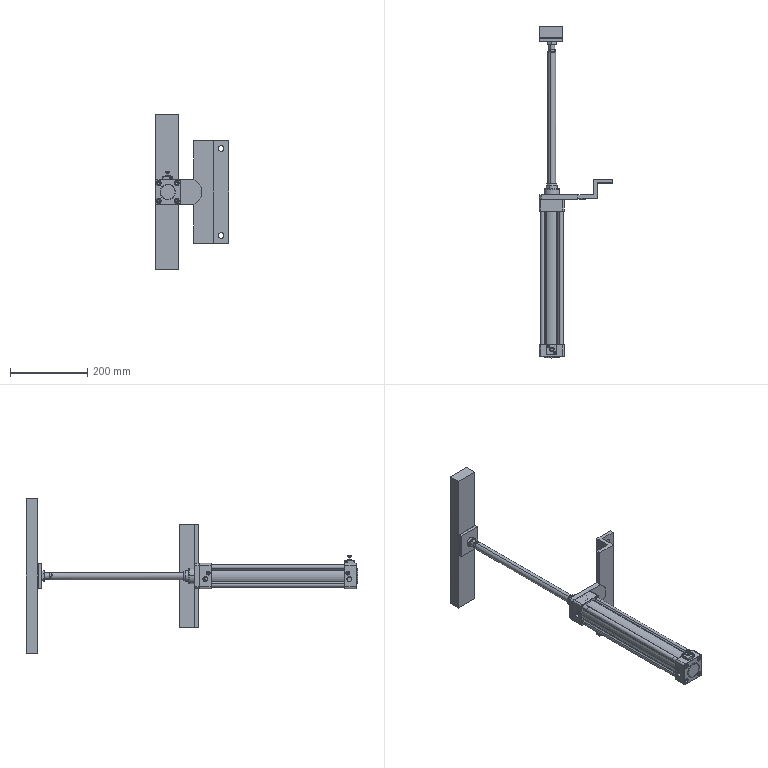Part | SolidWorks | features CompositeCurve 1 | 17 solids | 946 faces | box 190 x 856.5 x 400 mm | volume 1862385 mm3 | plane 379 | cylinder 265 | cone 240 | spline 62 | commonest cylinder face diameters 12 x32 8 x20 2 x16 6.647 x16 8.7 x16 12.7 x16